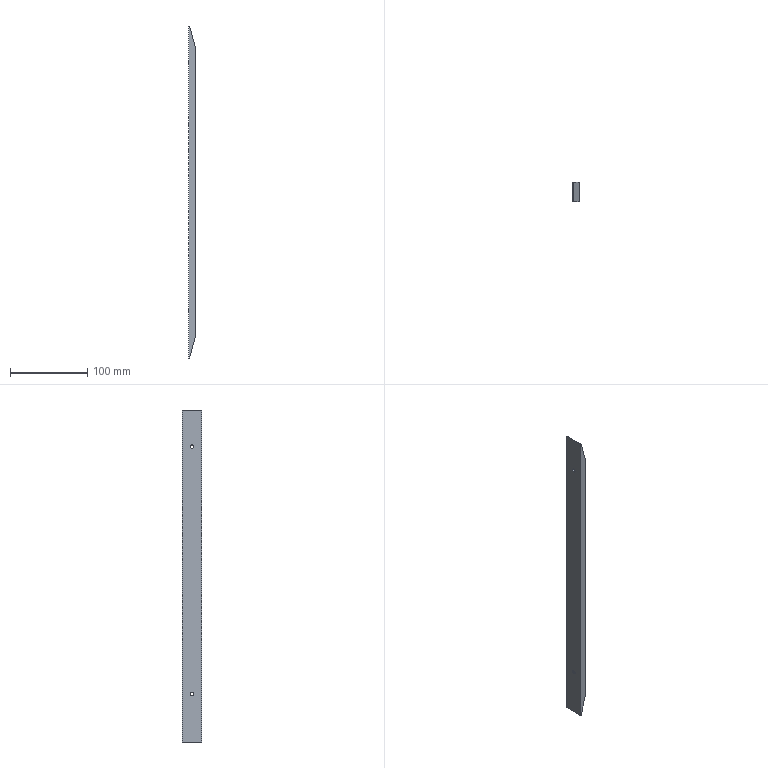Part | STEP file | 1 solid | 20 faces | box 8 x 25 x 430 mm | volume 80647 mm3 | plane 8 | cylinder 8 | cone 4 | commonest cylinder face diameters 4.5 x4 10 x4
STEP:
#1=CARTESIAN_POINT('',(0.,0.,0.));
#2=DIRECTION('',(0.,0.,1.));
#3=DIRECTION('',(1.,0.,0.));
#4=AXIS2_PLACEMENT_3D('',#1,#2,#3);
#5=CARTESIAN_POINT('',(47.75,-45.,-538.085));
#6=VERTEX_POINT('',#5);
#7=CARTESIAN_POINT('',(54.75,-45.,-511.961));
#8=VERTEX_POINT('',#7);
#9=CARTESIAN_POINT('',(47.75,-45.,-538.085));
#10=DIRECTION('',(0.2588,0.,0.9659));
#11=VECTOR('',#10,1.);
#12=LINE('',#9,#11);
#13=CARTESIAN_POINT('',(47.75,-70.,-538.085));
#14=DIRECTION('',(-0.9659,0.,0.2588));
#15=DIRECTION('',(0.,1.,0.));
#16=AXIS2_PLACEMENT_3D('',#13,#14,#15);
#17=PLANE('',#16);
#18=CARTESIAN_POINT('',(25.,0.));
#19=DIRECTION('',(0.,-1.));
#20=VECTOR('',#19,1.);
#21=LINE('',#18,#20);
#22=(GEOMETRIC_REPRESENTATION_CONTEXT(2)PARAMETRIC_REPRESENTATION_CONTEXT()REPRESENTATION_CONTEXT('',''));
#23=DEFINITIONAL_REPRESENTATION('',(#21),#22);
#24=PCURVE('',#17,#23);
#25=CARTESIAN_POINT('',(51.75,-45.,-2500.));
#26=DIRECTION('',(0.,1.,0.));
#27=DIRECTION('',(1.,0.,0.));
#28=AXIS2_PLACEMENT_3D('',#25,#26,#27);
#29=PLANE('',#28);
#30=CARTESIAN_POINT('',(-4.,-1961.915));
#31=DIRECTION('',(0.2588,-0.9659));
#32=VECTOR('',#31,1.);
#33=LINE('',#30,#32);
#34=(GEOMETRIC_REPRESENTATION_CONTEXT(2)PARAMETRIC_REPRESENTATION_CONTEXT()REPRESENTATION_CONTEXT('',''));
#35=DEFINITIONAL_REPRESENTATION('',(#33),#34);
#36=PCURVE('',#29,#35);
#37=SURFACE_CURVE('',#12,(#24,#36),.PCURVE_S1.);
#38=EDGE_CURVE('',#6,#8,#37,.T.);
#39=ORIENTED_EDGE('',*,*,#38,.T.);
#40=CARTESIAN_POINT('',(54.75,-70.,-511.961));
#41=VERTEX_POINT('',#40);
#42=CARTESIAN_POINT('',(54.75,-70.,-511.961));
#43=DIRECTION('',(0.,1.,0.));
#44=VECTOR('',#43,1.);
#45=LINE('',#42,#44);
#46=CARTESIAN_POINT('',(0.,-27.046));
#47=DIRECTION('',(1.,0.));
#48=VECTOR('',#47,1.);
#49=LINE('',#46,#48);
#50=(GEOMETRIC_REPRESENTATION_CONTEXT(2)PARAMETRIC_REPRESENTATION_CONTEXT()REPRESENTATION_CONTEXT('',''));
#51=DEFINITIONAL_REPRESENTATION('',(#49),#50);
#52=PCURVE('',#17,#51);
#53=CARTESIAN_POINT('',(54.75,0.,0.));
#54=DIRECTION('',(1.,0.,0.));
#55=DIRECTION('',(0.,1.,0.));
#56=AXIS2_PLACEMENT_3D('',#53,#54,#55);
#57=PLANE('',#56);
#58=CARTESIAN_POINT('',(-70.,-511.961));
#59=DIRECTION('',(1.,0.));
#60=VECTOR('',#59,1.);
#61=LINE('',#58,#60);
#62=(GEOMETRIC_REPRESENTATION_CONTEXT(2)PARAMETRIC_REPRESENTATION_CONTEXT()REPRESENTATION_CONTEXT('',''));
#63=DEFINITIONAL_REPRESENTATION('',(#61),#62);
#64=PCURVE('',#57,#63);
#65=SURFACE_CURVE('',#45,(#52,#64),.PCURVE_S1.);
#66=EDGE_CURVE('',#41,#8,#65,.T.);
#67=ORIENTED_EDGE('',*,*,#66,.F.);
#68=CARTESIAN_POINT('',(47.75,-70.,-538.085));
#69=VERTEX_POINT('',#68);
#70=CARTESIAN_POINT('',(47.75,-70.,-538.085));
#71=DIRECTION('',(0.2588,0.,0.9659));
#72=VECTOR('',#71,1.);
#73=LINE('',#70,#72);
#74=CARTESIAN_POINT('',(0.,0.));
#75=DIRECTION('',(0.,-1.));
#76=VECTOR('',#75,1.);
#77=LINE('',#74,#76);
#78=(GEOMETRIC_REPRESENTATION_CONTEXT(2)PARAMETRIC_REPRESENTATION_CONTEXT()REPRESENTATION_CONTEXT('',''));
#79=DEFINITIONAL_REPRESENTATION('',(#77),#78);
#80=PCURVE('',#17,#79);
#81=CARTESIAN_POINT('',(51.75,-70.,-2500.));
#82=DIRECTION('',(0.,-1.,0.));
#83=DIRECTION('',(0.,0.,-1.));
#84=AXIS2_PLACEMENT_3D('',#81,#82,#83);
#85=PLANE('',#84);
#86=CARTESIAN_POINT('',(-1961.915,-4.));
#87=DIRECTION('',(-0.9659,0.2588));
#88=VECTOR('',#87,1.);
#89=LINE('',#86,#88);
#90=(GEOMETRIC_REPRESENTATION_CONTEXT(2)PARAMETRIC_REPRESENTATION_CONTEXT()REPRESENTATION_CONTEXT('',''));
#91=DEFINITIONAL_REPRESENTATION('',(#89),#90);
#92=PCURVE('',#85,#91);
#93=SURFACE_CURVE('',#73,(#80,#92),.PCURVE_S1.);
#94=EDGE_CURVE('',#69,#41,#93,.T.);
#95=ORIENTED_EDGE('',*,*,#94,.F.);
#96=CARTESIAN_POINT('',(47.75,-70.,-538.085));
#97=DIRECTION('',(0.,1.,0.));
#98=VECTOR('',#97,1.);
#99=LINE('',#96,#98);
#100=CARTESIAN_POINT('',(0.,0.));
#101=DIRECTION('',(1.,0.));
#102=VECTOR('',#101,1.);
#103=LINE('',#100,#102);
#104=(GEOMETRIC_REPRESENTATION_CONTEXT(2)PARAMETRIC_REPRESENTATION_CONTEXT()REPRESENTATION_CONTEXT('',''));
#105=DEFINITIONAL_REPRESENTATION('',(#103),#104);
#106=PCURVE('',#17,#105);
#107=CARTESIAN_POINT('',(41.75,-45.,-538.085));
#108=DIRECTION('',(0.,0.,1.));
#109=DIRECTION('',(1.,0.,0.));
#110=AXIS2_PLACEMENT_3D('',#107,#108,#109);
#111=PLANE('',#110);
#112=CARTESIAN_POINT('',(6.,-25.));
#113=DIRECTION('',(0.,1.));
#114=VECTOR('',#113,1.);
#115=LINE('',#112,#114);
#116=(GEOMETRIC_REPRESENTATION_CONTEXT(2)PARAMETRIC_REPRESENTATION_CONTEXT()REPRESENTATION_CONTEXT('',''));
#117=DEFINITIONAL_REPRESENTATION('',(#115),#116);
#118=PCURVE('',#111,#117);
#119=SURFACE_CURVE('',#99,(#106,#118),.PCURVE_S1.);
#120=EDGE_CURVE('',#69,#6,#119,.T.);
#121=ORIENTED_EDGE('',*,*,#120,.T.);
#122=EDGE_LOOP('',(#39,#67,#95,#121));
#123=FACE_BOUND('',#122,.T.);
#124=ADVANCED_FACE('',(#123),#17,.F.);
#125=CARTESIAN_POINT('',(54.75,-45.,-134.21));
#126=VERTEX_POINT('',#125);
#127=CARTESIAN_POINT('',(47.75,-45.,-108.085));
#128=VERTEX_POINT('',#127);
#129=CARTESIAN_POINT('',(47.75,-45.,-108.085));
#130=DIRECTION('',(-0.2588,0.,0.9659));
#131=VECTOR('',#130,1.);
#132=LINE('',#129,#131);
#133=CARTESIAN_POINT('',(47.75,-70.,-108.085));
#134=DIRECTION('',(-0.9659,0.,-0.2588));
#135=DIRECTION('',(-0.2588,0.,0.9659));
#136=AXIS2_PLACEMENT_3D('',#133,#134,#135);
#137=PLANE('',#136);
#138=CARTESIAN_POINT('',(0.,25.));
#139=DIRECTION('',(1.,0.));
#140=VECTOR('',#139,1.);
#141=LINE('',#138,#140);
#142=(GEOMETRIC_REPRESENTATION_CONTEXT(2)PARAMETRIC_REPRESENTATION_CONTEXT()REPRESENTATION_CONTEXT('',''));
#143=DEFINITIONAL_REPRESENTATION('',(#141),#142);
#144=PCURVE('',#137,#143);
#145=CARTESIAN_POINT('',(-4.,-2391.915));
#146=DIRECTION('',(-0.2588,-0.9659));
#147=VECTOR('',#146,1.);
#148=LINE('',#145,#147);
#149=(GEOMETRIC_REPRESENTATION_CONTEXT(2)PARAMETRIC_REPRESENTATION_CONTEXT()REPRESENTATION_CONTEXT('',''));
#150=DEFINITIONAL_REPRESENTATION('',(#148),#149);
#151=PCURVE('',#29,#150);
#152=SURFACE_CURVE('',#132,(#144,#151),.PCURVE_S1.);
#153=EDGE_CURVE('',#126,#128,#152,.T.);
#154=ORIENTED_EDGE('',*,*,#153,.T.);
#155=CARTESIAN_POINT('',(47.75,-70.,-108.085));
#156=VERTEX_POINT('',#155);
#157=CARTESIAN_POINT('',(47.75,-70.,-108.085));
#158=DIRECTION('',(0.,1.,0.));
#159=VECTOR('',#158,1.);
#160=LINE('',#157,#159);
#161=CARTESIAN_POINT('',(0.,0.));
#162=DIRECTION('',(0.,1.));
#163=VECTOR('',#162,1.);
#164=LINE('',#161,#163);
#165=(GEOMETRIC_REPRESENTATION_CONTEXT(2)PARAMETRIC_REPRESENTATION_CONTEXT()REPRESENTATION_CONTEXT('',''));
#166=DEFINITIONAL_REPRESENTATION('',(#164),#165);
#167=PCURVE('',#137,#166);
#168=CARTESIAN_POINT('',(41.75,-45.,-108.085));
#169=DIRECTION('',(0.,0.,-1.));
#170=DIRECTION('',(0.,-1.,0.));
#171=AXIS2_PLACEMENT_3D('',#168,#169,#170);
#172=PLANE('',#171);
#173=CARTESIAN_POINT('',(25.,-6.));
#174=DIRECTION('',(-1.,0.));
#175=VECTOR('',#174,1.);
#176=LINE('',#173,#175);
#177=(GEOMETRIC_REPRESENTATION_CONTEXT(2)PARAMETRIC_REPRESENTATION_CONTEXT()REPRESENTATION_CONTEXT('',''));
#178=DEFINITIONAL_REPRESENTATION('',(#176),#177);
#179=PCURVE('',#172,#178);
#180=SURFACE_CURVE('',#160,(#167,#179),.PCURVE_S1.);
#181=EDGE_CURVE('',#156,#128,#180,.T.);
#182=ORIENTED_EDGE('',*,*,#181,.F.);
#183=CARTESIAN_POINT('',(54.75,-70.,-134.21));
#184=VERTEX_POINT('',#183);
#185=CARTESIAN_POINT('',(47.75,-70.,-108.085));
#186=DIRECTION('',(-0.2588,0.,0.9659));
#187=VECTOR('',#186,1.);
#188=LINE('',#185,#187);
#189=CARTESIAN_POINT('',(0.,0.));
#190=DIRECTION('',(1.,0.));
#191=VECTOR('',#190,1.);
#192=LINE('',#189,#191);
#193=(GEOMETRIC_REPRESENTATION_CONTEXT(2)PARAMETRIC_REPRESENTATION_CONTEXT()REPRESENTATION_CONTEXT('',''));
#194=DEFINITIONAL_REPRESENTATION('',(#192),#193);
#195=PCURVE('',#137,#194);
#196=CARTESIAN_POINT('',(-2391.915,-4.));
#197=DIRECTION('',(-0.9659,-0.2588));
#198=VECTOR('',#197,1.);
#199=LINE('',#196,#198);
#200=(GEOMETRIC_REPRESENTATION_CONTEXT(2)PARAMETRIC_REPRESENTATION_CONTEXT()REPRESENTATION_CONTEXT('',''));
#201=DEFINITIONAL_REPRESENTATION('',(#199),#200);
#202=PCURVE('',#85,#201);
#203=SURFACE_CURVE('',#188,(#195,#202),.PCURVE_S1.);
#204=EDGE_CURVE('',#184,#156,#203,.T.);
#205=ORIENTED_EDGE('',*,*,#204,.F.);
#206=CARTESIAN_POINT('',(54.75,-70.,-134.21));
#207=DIRECTION('',(0.,1.,0.));
#208=VECTOR('',#207,1.);
#209=LINE('',#206,#208);
#210=CARTESIAN_POINT('',(-27.046,0.));
#211=DIRECTION('',(0.,1.));
#212=VECTOR('',#211,1.);
#213=LINE('',#210,#212);
#214=(GEOMETRIC_REPRESENTATION_CONTEXT(2)PARAMETRIC_REPRESENTATION_CONTEXT()REPRESENTATION_CONTEXT('',''));
#215=DEFINITIONAL_REPRESENTATION('',(#213),#214);
#216=PCURVE('',#137,#215);
#217=CARTESIAN_POINT('',(-70.,-134.21));
#218=DIRECTION('',(1.,0.));
#219=VECTOR('',#218,1.);
#220=LINE('',#217,#219);
#221=(GEOMETRIC_REPRESENTATION_CONTEXT(2)PARAMETRIC_REPRESENTATION_CONTEXT()REPRESENTATION_CONTEXT('',''));
#222=DEFINITIONAL_REPRESENTATION('',(#220),#221);
#223=PCURVE('',#57,#222);
#224=SURFACE_CURVE('',#209,(#216,#223),.PCURVE_S1.);
#225=EDGE_CURVE('',#184,#126,#224,.T.);
#226=ORIENTED_EDGE('',*,*,#225,.T.);
#227=EDGE_LOOP('',(#154,#182,#205,#226));
#228=FACE_BOUND('',#227,.T.);
#229=ADVANCED_FACE('',(#228),#137,.F.);
#230=CARTESIAN_POINT('',(51.75,-57.5,-480.585));
#231=VERTEX_POINT('',#230);
#232=CARTESIAN_POINT('',(51.75,-57.5,-470.585));
#233=VERTEX_POINT('',#232);
#234=CARTESIAN_POINT('',(51.75,-57.5,-475.585));
#235=DIRECTION('',(1.,0.,0.));
#236=DIRECTION('',(0.,0.,-1.));
#237=AXIS2_PLACEMENT_3D('',#234,#235,#236);
#238=CIRCLE('',#237,5.);
#239=CARTESIAN_POINT('',(54.75,-57.5,-475.585));
#240=DIRECTION('',(-1.,0.,0.));
#241=DIRECTION('',(0.,0.,1.));
#242=AXIS2_PLACEMENT_3D('',#239,#240,#241);
#243=CYLINDRICAL_SURFACE('',#242,5.);
#244=CARTESIAN_POINT('',(3.142,3.));
#245=DIRECTION('',(-1.,0.));
#246=VECTOR('',#245,1.);
#247=LINE('',#244,#246);
#248=(GEOMETRIC_REPRESENTATION_CONTEXT(2)PARAMETRIC_REPRESENTATION_CONTEXT()REPRESENTATION_CONTEXT('',''));
#249=DEFINITIONAL_REPRESENTATION('',(#247),#248);
#250=PCURVE('',#243,#249);
#251=CARTESIAN_POINT('',(51.75,-57.5,-475.585));
#252=DIRECTION('',(1.,0.,0.));
#253=DIRECTION('',(0.,0.,-1.));
#254=AXIS2_PLACEMENT_3D('',#251,#252,#253);
#255=CONICAL_SURFACE('',#254,5.,0.7854);
#256=CARTESIAN_POINT('',(0.,0.));
#257=DIRECTION('',(1.,0.));
#258=VECTOR('',#257,1.);
#259=LINE('',#256,#258);
#260=(GEOMETRIC_REPRESENTATION_CONTEXT(2)PARAMETRIC_REPRESENTATION_CONTEXT()REPRESENTATION_CONTEXT('',''));
#261=DEFINITIONAL_REPRESENTATION('',(#259),#260);
#262=PCURVE('',#255,#261);
#263=SURFACE_CURVE('',#238,(#250,#262),.PCURVE_S1.);
#264=EDGE_CURVE('',#231,#233,#263,.T.);
#265=ORIENTED_EDGE('',*,*,#264,.T.);
#266=CARTESIAN_POINT('',(54.75,-57.5,-470.585));
#267=VERTEX_POINT('',#266);
#268=CARTESIAN_POINT('',(54.75,-57.5,-470.585));
#269=DIRECTION('',(-1.,0.,0.));
#270=VECTOR('',#269,1.);
#271=LINE('',#268,#270);
#272=CARTESIAN_POINT('',(0.,0.));
#273=DIRECTION('',(0.,1.));
#274=VECTOR('',#273,1.);
#275=LINE('',#272,#274);
#276=(GEOMETRIC_REPRESENTATION_CONTEXT(2)PARAMETRIC_REPRESENTATION_CONTEXT()REPRESENTATION_CONTEXT('',''));
#277=DEFINITIONAL_REPRESENTATION('',(#275),#276);
#278=PCURVE('',#243,#277);
#279=CARTESIAN_POINT('',(54.75,-57.5,-475.585));
#280=DIRECTION('',(-1.,0.,0.));
#281=DIRECTION('',(0.,0.,1.));
#282=AXIS2_PLACEMENT_3D('',#279,#280,#281);
#283=CYLINDRICAL_SURFACE('',#282,5.);
#284=CARTESIAN_POINT('',(6.283,0.));
#285=DIRECTION('',(0.,1.));
#286=VECTOR('',#285,1.);
#287=LINE('',#284,#286);
#288=(GEOMETRIC_REPRESENTATION_CONTEXT(2)PARAMETRIC_REPRESENTATION_CONTEXT()REPRESENTATION_CONTEXT('',''));
#289=DEFINITIONAL_REPRESENTATION('',(#287),#288);
#290=PCURVE('',#283,#289);
#291=SURFACE_CURVE('',#271,(#278,#290),.PCURVE_S1.);
#292=EDGE_CURVE('',#267,#233,#291,.T.);
#293=ORIENTED_EDGE('',*,*,#292,.F.);
#294=CARTESIAN_POINT('',(54.75,-57.5,-480.585));
#295=VERTEX_POINT('',#294);
#296=CARTESIAN_POINT('',(54.75,-57.5,-475.585));
#297=DIRECTION('',(1.,0.,0.));
#298=DIRECTION('',(0.,0.,-1.));
#299=AXIS2_PLACEMENT_3D('',#296,#297,#298);
#300=CIRCLE('',#299,5.);
#301=CARTESIAN_POINT('',(3.142,0.));
#302=DIRECTION('',(-1.,0.));
#303=VECTOR('',#302,1.);
#304=LINE('',#301,#303);
#305=(GEOMETRIC_REPRESENTATION_CONTEXT(2)PARAMETRIC_REPRESENTATION_CONTEXT()REPRESENTATION_CONTEXT('',''));
#306=DEFINITIONAL_REPRESENTATION('',(#304),#305);
#307=PCURVE('',#243,#306);
#308=CARTESIAN_POINT('',(-57.5,-475.585));
#309=DIRECTION('',(0.,-1.));
#310=AXIS2_PLACEMENT_2D('',#308,#309);
#311=CIRCLE('',#310,5.);
#312=(GEOMETRIC_REPRESENTATION_CONTEXT(2)PARAMETRIC_REPRESENTATION_CONTEXT()REPRESENTATION_CONTEXT('',''));
#313=DEFINITIONAL_REPRESENTATION('',(#311),#312);
#314=PCURVE('',#57,#313);
#315=SURFACE_CURVE('',#300,(#307,#314),.PCURVE_S1.);
#316=EDGE_CURVE('',#295,#267,#315,.T.);
#317=ORIENTED_EDGE('',*,*,#316,.F.);
#318=CARTESIAN_POINT('',(54.75,-57.5,-480.585));
#319=DIRECTION('',(-1.,0.,0.));
#320=VECTOR('',#319,1.);
#321=LINE('',#318,#320);
#322=CARTESIAN_POINT('',(3.142,0.));
#323=DIRECTION('',(0.,1.));
#324=VECTOR('',#323,1.);
#325=LINE('',#322,#324);
#326=(GEOMETRIC_REPRESENTATION_CONTEXT(2)PARAMETRIC_REPRESENTATION_CONTEXT()REPRESENTATION_CONTEXT('',''));
#327=DEFINITIONAL_REPRESENTATION('',(#325),#326);
#328=PCURVE('',#243,#327);
#329=CARTESIAN_POINT('',(3.142,0.));
#330=DIRECTION('',(0.,1.));
#331=VECTOR('',#330,1.);
#332=LINE('',#329,#331);
#333=(GEOMETRIC_REPRESENTATION_CONTEXT(2)PARAMETRIC_REPRESENTATION_CONTEXT()REPRESENTATION_CONTEXT('',''));
#334=DEFINITIONAL_REPRESENTATION('',(#332),#333);
#335=PCURVE('',#283,#334);
#336=SURFACE_CURVE('',#321,(#328,#335),.PCURVE_S1.);
#337=EDGE_CURVE('',#295,#231,#336,.T.);
#338=ORIENTED_EDGE('',*,*,#337,.T.);
#339=EDGE_LOOP('',(#265,#293,#317,#338));
#340=FACE_BOUND('',#339,.F.);
#341=ADVANCED_FACE('',(#340),#243,.F.);
#342=CARTESIAN_POINT('',(51.75,-57.5,-160.585));
#343=VERTEX_POINT('',#342);
#344=CARTESIAN_POINT('',(51.75,-57.5,-150.585));
#345=VERTEX_POINT('',#344);
#346=CARTESIAN_POINT('',(51.75,-57.5,-155.585));
#347=DIRECTION('',(1.,0.,0.));
#348=DIRECTION('',(0.,0.,-1.));
#349=AXIS2_PLACEMENT_3D('',#346,#347,#348);
#350=CIRCLE('',#349,5.);
#351=CARTESIAN_POINT('',(54.75,-57.5,-155.585));
#352=DIRECTION('',(-1.,0.,0.));
#353=DIRECTION('',(0.,0.,1.));
#354=AXIS2_PLACEMENT_3D('',#351,#352,#353);
#355=CYLINDRICAL_SURFACE('',#354,5.);
#356=CARTESIAN_POINT('',(3.142,3.));
#357=DIRECTION('',(-1.,0.));
#358=VECTOR('',#357,1.);
#359=LINE('',#356,#358);
#360=(GEOMETRIC_REPRESENTATION_CONTEXT(2)PARAMETRIC_REPRESENTATION_CONTEXT()REPRESENTATION_CONTEXT('',''));
#361=DEFINITIONAL_REPRESENTATION('',(#359),#360);
#362=PCURVE('',#355,#361);
#363=CARTESIAN_POINT('',(51.75,-57.5,-155.585));
#364=DIRECTION('',(1.,0.,0.));
#365=DIRECTION('',(0.,0.,-1.));
#366=AXIS2_PLACEMENT_3D('',#363,#364,#365);
#367=CONICAL_SURFACE('',#366,5.,0.7854);
#368=CARTESIAN_POINT('',(0.,0.));
#369=DIRECTION('',(1.,0.));
#370=VECTOR('',#369,1.);
#371=LINE('',#368,#370);
#372=(GEOMETRIC_REPRESENTATION_CONTEXT(2)PARAMETRIC_REPRESENTATION_CONTEXT()REPRESENTATION_CONTEXT('',''));
#373=DEFINITIONAL_REPRESENTATION('',(#371),#372);
#374=PCURVE('',#367,#373);
#375=SURFACE_CURVE('',#350,(#362,#374),.PCURVE_S1.);
#376=EDGE_CURVE('',#343,#345,#375,.T.);
#377=ORIENTED_EDGE('',*,*,#376,.T.);
#378=CARTESIAN_POINT('',(54.75,-57.5,-150.585));
#379=VERTEX_POINT('',#378);
#380=CARTESIAN_POINT('',(54.75,-57.5,-150.585));
#381=DIRECTION('',(-1.,0.,0.));
#382=VECTOR('',#381,1.);
#383=LINE('',#380,#382);
#384=CARTESIAN_POINT('',(0.,0.));
#385=DIRECTION('',(0.,1.));
#386=VECTOR('',#385,1.);
#387=LINE('',#384,#386);
#388=(GEOMETRIC_REPRESENTATION_CONTEXT(2)PARAMETRIC_REPRESENTATION_CONTEXT()REPRESENTATION_CONTEXT('',''));
#389=DEFINITIONAL_REPRESENTATION('',(#387),#388);
#390=PCURVE('',#355,#389);
#391=CARTESIAN_POINT('',(54.75,-57.5,-155.585));
#392=DIRECTION('',(-1.,0.,0.));
#393=DIRECTION('',(0.,0.,1.));
#394=AXIS2_PLACEMENT_3D('',#391,#392,#393);
#395=CYLINDRICAL_SURFACE('',#394,5.);
#396=CARTESIAN_POINT('',(6.283,0.));
#397=DIRECTION('',(0.,1.));
#398=VECTOR('',#397,1.);
#399=LINE('',#396,#398);
#400=(GEOMETRIC_REPRESENTATION_CONTEXT(2)PARAMETRIC_REPRESENTATION_CONTEXT()REPRESENTATION_CONTEXT('',''));
#401=DEFINITIONAL_REPRESENTATION('',(#399),#400);
#402=PCURVE('',#395,#401);
#403=SURFACE_CURVE('',#383,(#390,#402),.PCURVE_S1.);
#404=EDGE_CURVE('',#379,#345,#403,.T.);
#405=ORIENTED_EDGE('',*,*,#404,.F.);
#406=CARTESIAN_POINT('',(54.75,-57.5,-160.585));
#407=VERTEX_POINT('',#406);
#408=CARTESIAN_POINT('',(54.75,-57.5,-155.585));
#409=DIRECTION('',(1.,0.,0.));
#410=DIRECTION('',(0.,0.,-1.));
#411=AXIS2_PLACEMENT_3D('',#408,#409,#410);
#412=CIRCLE('',#411,5.);
#413=CARTESIAN_POINT('',(3.142,0.));
#414=DIRECTION('',(-1.,0.));
#415=VECTOR('',#414,1.);
#416=LINE('',#413,#415);
#417=(GEOMETRIC_REPRESENTATION_CONTEXT(2)PARAMETRIC_REPRESENTATION_CONTEXT()REPRESENTATION_CONTEXT('',''));
#418=DEFINITIONAL_REPRESENTATION('',(#416),#417);
#419=PCURVE('',#355,#418);
#420=CARTESIAN_POINT('',(-57.5,-155.585));
#421=DIRECTION('',(0.,-1.));
#422=AXIS2_PLACEMENT_2D('',#420,#421);
#423=CIRCLE('',#422,5.);
#424=(GEOMETRIC_REPRESENTATION_CONTEXT(2)PARAMETRIC_REPRESENTATION_CONTEXT()REPRESENTATION_CONTEXT('',''));
#425=DEFINITIONAL_REPRESENTATION('',(#423),#424);
#426=PCURVE('',#57,#425);
#427=SURFACE_CURVE('',#412,(#419,#426),.PCURVE_S1.);
#428=EDGE_CURVE('',#407,#379,#427,.T.);
#429=ORIENTED_EDGE('',*,*,#428,.F.);
#430=CARTESIAN_POINT('',(54.75,-57.5,-160.585));
#431=DIRECTION('',(-1.,0.,0.));
#432=VECTOR('',#431,1.);
#433=LINE('',#430,#432);
#434=CARTESIAN_POINT('',(3.142,0.));
#435=DIRECTION('',(0.,1.));
#436=VECTOR('',#435,1.);
#437=LINE('',#434,#436);
#438=(GEOMETRIC_REPRESENTATION_CONTEXT(2)PARAMETRIC_REPRESENTATION_CONTEXT()REPRESENTATION_CONTEXT('',''));
#439=DEFINITIONAL_REPRESENTATION('',(#437),#438);
#440=PCURVE('',#355,#439);
#441=CARTESIAN_POINT('',(3.142,0.));
#442=DIRECTION('',(0.,1.));
#443=VECTOR('',#442,1.);
#444=LINE('',#441,#443);
#445=(GEOMETRIC_REPRESENTATION_CONTEXT(2)PARAMETRIC_REPRESENTATION_CONTEXT()REPRESENTATION_CONTEXT('',''));
#446=DEFINITIONAL_REPRESENTATION('',(#444),#445);
#447=PCURVE('',#395,#446);
#448=SURFACE_CURVE('',#433,(#440,#447),.PCURVE_S1.);
#449=EDGE_CURVE('',#407,#343,#448,.T.);
#450=ORIENTED_EDGE('',*,*,#449,.T.);
#451=EDGE_LOOP('',(#377,#405,#429,#450));
#452=FACE_BOUND('',#451,.F.);
#453=ADVANCED_FACE('',(#452),#355,.F.);
#454=CARTESIAN_POINT('',(54.75,-57.5,-475.585));
#455=DIRECTION('',(1.,0.,0.));
#456=DIRECTION('',(0.,0.,-1.));
#457=AXIS2_PLACEMENT_3D('',#454,#455,#456);
#458=CIRCLE('',#457,5.);
#459=CARTESIAN_POINT('',(-57.5,-475.585));
#460=DIRECTION('',(0.,-1.));
#461=AXIS2_PLACEMENT_2D('',#459,#460);
#462=CIRCLE('',#461,5.);
#463=(GEOMETRIC_REPRESENTATION_CONTEXT(2)PARAMETRIC_REPRESENTATION_CONTEXT()REPRESENTATION_CONTEXT('',''));
#464=DEFINITIONAL_REPRESENTATION('',(#462),#463);
#465=PCURVE('',#57,#464);
#466=CARTESIAN_POINT('',(9.425,0.));
#467=DIRECTION('',(-1.,0.));
#468=VECTOR('',#467,1.);
#469=LINE('',#466,#468);
#470=(GEOMETRIC_REPRESENTATION_CONTEXT(2)PARAMETRIC_REPRESENTATION_CONTEXT()REPRESENTATION_CONTEXT('',''));
#471=DEFINITIONAL_REPRESENTATION('',(#469),#470);
#472=PCURVE('',#283,#471);
#473=SURFACE_CURVE('',#458,(#465,#472),.PCURVE_S1.);
#474=EDGE_CURVE('',#267,#295,#473,.T.);
#475=ORIENTED_EDGE('',*,*,#474,.F.);
#476=ORIENTED_EDGE('',*,*,#316,.F.);
#477=EDGE_LOOP('',(#475,#476));
#478=FACE_BOUND('',#477,.T.);
#479=CARTESIAN_POINT('',(54.75,-57.5,-155.585));
#480=DIRECTION('',(1.,0.,0.));
#481=DIRECTION('',(0.,0.,-1.));
#482=AXIS2_PLACEMENT_3D('',#479,#480,#481);
#483=CIRCLE('',#482,5.);
#484=CARTESIAN_POINT('',(-57.5,-155.585));
#485=DIRECTION('',(0.,-1.));
#486=AXIS2_PLACEMENT_2D('',#484,#485);
#487=CIRCLE('',#486,5.);
#488=(GEOMETRIC_REPRESENTATION_CONTEXT(2)PARAMETRIC_REPRESENTATION_CONTEXT()REPRESENTATION_CONTEXT('',''));
#489=DEFINITIONAL_REPRESENTATION('',(#487),#488);
#490=PCURVE('',#57,#489);
#491=CARTESIAN_POINT('',(9.425,0.));
#492=DIRECTION('',(-1.,0.));
#493=VECTOR('',#492,1.);
#494=LINE('',#491,#493);
#495=(GEOMETRIC_REPRESENTATION_CONTEXT(2)PARAMETRIC_REPRESENTATION_CONTEXT()REPRESENTATION_CONTEXT('',''));
#496=DEFINITIONAL_REPRESENTATION('',(#494),#495);
#497=PCURVE('',#395,#496);
#498=SURFACE_CURVE('',#483,(#490,#497),.PCURVE_S1.);
#499=EDGE_CURVE('',#379,#407,#498,.T.);
#500=ORIENTED_EDGE('',*,*,#499,.F.);
#501=ORIENTED_EDGE('',*,*,#428,.F.);
#502=EDGE_LOOP('',(#500,#501));
#503=FACE_BOUND('',#502,.T.);
#504=ORIENTED_EDGE('',*,*,#66,.T.);
#505=CARTESIAN_POINT('',(54.75,-45.,-558.085));
#506=DIRECTION('',(0.,0.,1.));
#507=VECTOR('',#506,1.);
#508=LINE('',#505,#507);
#509=CARTESIAN_POINT('',(-45.,-558.085));
#510=DIRECTION('',(0.,1.));
#511=VECTOR('',#510,1.);
#512=LINE('',#509,#511);
#513=(GEOMETRIC_REPRESENTATION_CONTEXT(2)PARAMETRIC_REPRESENTATION_CONTEXT()REPRESENTATION_CONTEXT('',''));
#514=DEFINITIONAL_REPRESENTATION('',(#512),#513);
#515=PCURVE('',#57,#514);
#516=CARTESIAN_POINT('',(3.,-1941.915));
#517=DIRECTION('',(0.,-1.));
#518=VECTOR('',#517,1.);
#519=LINE('',#516,#518);
#520=(GEOMETRIC_REPRESENTATION_CONTEXT(2)PARAMETRIC_REPRESENTATION_CONTEXT()REPRESENTATION_CONTEXT('',''));
#521=DEFINITIONAL_REPRESENTATION('',(#519),#520);
#522=PCURVE('',#29,#521);
#523=SURFACE_CURVE('',#508,(#515,#522),.PCURVE_S1.);
#524=EDGE_CURVE('',#8,#126,#523,.T.);
#525=ORIENTED_EDGE('',*,*,#524,.T.);
#526=ORIENTED_EDGE('',*,*,#225,.F.);
#527=CARTESIAN_POINT('',(54.75,-70.,-108.085));
#528=DIRECTION('',(0.,0.,-1.));
#529=VECTOR('',#528,1.);
#530=LINE('',#527,#529);
#531=CARTESIAN_POINT('',(-70.,-108.085));
#532=DIRECTION('',(0.,-1.));
#533=VECTOR('',#532,1.);
#534=LINE('',#531,#533);
#535=(GEOMETRIC_REPRESENTATION_CONTEXT(2)PARAMETRIC_REPRESENTATION_CONTEXT()REPRESENTATION_CONTEXT('',''));
#536=DEFINITIONAL_REPRESENTATION('',(#534),#535);
#537=PCURVE('',#57,#536);
#538=CARTESIAN_POINT('',(-2391.915,3.));
#539=DIRECTION('',(1.,0.));
#540=VECTOR('',#539,1.);
#541=LINE('',#538,#540);
#542=(GEOMETRIC_REPRESENTATION_CONTEXT(2)PARAMETRIC_REPRESENTATION_CONTEXT()REPRESENTATION_CONTEXT('',''));
#543=DEFINITIONAL_REPRESENTATION('',(#541),#542);
#544=PCURVE('',#85,#543);
#545=SURFACE_CURVE('',#530,(#537,#544),.PCURVE_S1.);
#546=EDGE_CURVE('',#184,#41,#545,.T.);
#547=ORIENTED_EDGE('',*,*,#546,.T.);
#548=EDGE_LOOP('',(#504,#525,#526,#547));
#549=FACE_BOUND('',#548,.T.);
#550=ADVANCED_FACE('',(#478,#503,#549),#57,.T.);
#551=ORIENTED_EDGE('',*,*,#264,.F.);
#552=CARTESIAN_POINT('',(49.,-57.5,-477.835));
#553=VERTEX_POINT('',#552);
#554=CARTESIAN_POINT('',(51.75,-57.5,-480.585));
#555=DIRECTION('',(0.7071,0.,-0.7071));
#556=VECTOR('',#555,1.);
#557=LINE('',#554,#556);
#558=CARTESIAN_POINT('',(0.,0.));
#559=DIRECTION('',(0.,1.));
#560=VECTOR('',#559,1.);
#561=LINE('',#558,#560);
#562=(GEOMETRIC_REPRESENTATION_CONTEXT(2)PARAMETRIC_REPRESENTATION_CONTEXT()REPRESENTATION_CONTEXT('',''));
#563=DEFINITIONAL_REPRESENTATION('',(#561),#562);
#564=PCURVE('',#255,#563);
#565=CARTESIAN_POINT('',(51.75,-57.5,-475.585));
#566=DIRECTION('',(1.,0.,0.));
#567=DIRECTION('',(0.,0.,-1.));
#568=AXIS2_PLACEMENT_3D('',#565,#566,#567);
#569=CONICAL_SURFACE('',#568,5.,0.7854);
#570=CARTESIAN_POINT('',(6.283,0.));
#571=DIRECTION('',(0.,1.));
#572=VECTOR('',#571,1.);
#573=LINE('',#570,#572);
#574=(GEOMETRIC_REPRESENTATION_CONTEXT(2)PARAMETRIC_REPRESENTATION_CONTEXT()REPRESENTATION_CONTEXT('',''));
#575=DEFINITIONAL_REPRESENTATION('',(#573),#574);
#576=PCURVE('',#569,#575);
#577=SURFACE_CURVE('',#557,(#564,#576),.PCURVE_S1.);
#578=EDGE_CURVE('',#553,#231,#577,.T.);
#579=ORIENTED_EDGE('',*,*,#578,.F.);
#580=CARTESIAN_POINT('',(49.,-57.5,-473.335));
#581=VERTEX_POINT('',#580);
#582=CARTESIAN_POINT('',(49.,-57.5,-475.585));
#583=DIRECTION('',(1.,0.,0.));
#584=DIRECTION('',(0.,0.,-1.));
#585=AXIS2_PLACEMENT_3D('',#582,#583,#584);
#586=CIRCLE('',#585,2.25);
#587=CARTESIAN_POINT('',(0.,-2.75));
#588=DIRECTION('',(1.,0.));
#589=VECTOR('',#588,1.);
#590=LINE('',#587,#589);
#591=(GEOMETRIC_REPRESENTATION_CONTEXT(2)PARAMETRIC_REPRESENTATION_CONTEXT()REPRESENTATION_CONTEXT('',''));
#592=DEFINITIONAL_REPRESENTATION('',(#590),#591);
#593=PCURVE('',#255,#592);
#594=CARTESIAN_POINT('',(51.75,-57.5,-475.585));
#595=DIRECTION('',(1.,0.,0.));
#596=DIRECTION('',(0.,0.,-1.));
#597=AXIS2_PLACEMENT_3D('',#594,#595,#596);
#598=CYLINDRICAL_SURFACE('',#597,2.25);
#599=CARTESIAN_POINT('',(0.,-2.75));
#600=DIRECTION('',(1.,0.));
#601=VECTOR('',#600,1.);
#602=LINE('',#599,#601);
#603=(GEOMETRIC_REPRESENTATION_CONTEXT(2)PARAMETRIC_REPRESENTATION_CONTEXT()REPRESENTATION_CONTEXT('',''));
#604=DEFINITIONAL_REPRESENTATION('',(#602),#603);
#605=PCURVE('',#598,#604);
#606=SURFACE_CURVE('',#586,(#593,#605),.PCURVE_S1.);
#607=EDGE_CURVE('',#553,#581,#606,.T.);
#608=ORIENTED_EDGE('',*,*,#607,.T.);
#609=CARTESIAN_POINT('',(51.75,-57.5,-470.585));
#610=DIRECTION('',(0.7071,0.,0.7071));
#611=VECTOR('',#610,1.);
#612=LINE('',#609,#611);
#613=CARTESIAN_POINT('',(3.142,0.));
#614=DIRECTION('',(0.,1.));
#615=VECTOR('',#614,1.);
#616=LINE('',#613,#615);
#617=(GEOMETRIC_REPRESENTATION_CONTEXT(2)PARAMETRIC_REPRESENTATION_CONTEXT()REPRESENTATION_CONTEXT('',''));
#618=DEFINITIONAL_REPRESENTATION('',(#616),#617);
#619=PCURVE('',#255,#618);
#620=CARTESIAN_POINT('',(3.142,0.));
#621=DIRECTION('',(0.,1.));
#622=VECTOR('',#621,1.);
#623=LINE('',#620,#622);
#624=(GEOMETRIC_REPRESENTATION_CONTEXT(2)PARAMETRIC_REPRESENTATION_CONTEXT()REPRESENTATION_CONTEXT('',''));
#625=DEFINITIONAL_REPRESENTATION('',(#623),#624);
#626=PCURVE('',#569,#625);
#627=SURFACE_CURVE('',#612,(#619,#626),.PCURVE_S1.);
#628=EDGE_CURVE('',#581,#233,#627,.T.);
#629=ORIENTED_EDGE('',*,*,#628,.T.);
#630=EDGE_LOOP('',(#551,#579,#608,#629));
#631=FACE_BOUND('',#630,.F.);
#632=ADVANCED_FACE('',(#631),#255,.F.);
#633=ORIENTED_EDGE('',*,*,#607,.F.);
#634=CARTESIAN_POINT('',(46.75,-57.5,-477.835));
#635=VERTEX_POINT('',#634);
#636=CARTESIAN_POINT('',(51.75,-57.5,-477.835));
#637=DIRECTION('',(1.,0.,0.));
#638=VECTOR('',#637,1.);
#639=LINE('',#636,#638);
#640=CARTESIAN_POINT('',(0.,0.));
#641=DIRECTION('',(0.,1.));
#642=VECTOR('',#641,1.);
#643=LINE('',#640,#642);
#644=(GEOMETRIC_REPRESENTATION_CONTEXT(2)PARAMETRIC_REPRESENTATION_CONTEXT()REPRESENTATION_CONTEXT('',''));
#645=DEFINITIONAL_REPRESENTATION('',(#643),#644);
#646=PCURVE('',#598,#645);
#647=CARTESIAN_POINT('',(51.75,-57.5,-475.585));
#648=DIRECTION('',(1.,0.,0.));
#649=DIRECTION('',(0.,0.,-1.));
#650=AXIS2_PLACEMENT_3D('',#647,#648,#649);
#651=CYLINDRICAL_SURFACE('',#650,2.25);
#652=CARTESIAN_POINT('',(6.283,0.));
#653=DIRECTION('',(0.,1.));
#654=VECTOR('',#653,1.);
#655=LINE('',#652,#654);
#656=(GEOMETRIC_REPRESENTATION_CONTEXT(2)PARAMETRIC_REPRESENTATION_CONTEXT()REPRESENTATION_CONTEXT('',''));
#657=DEFINITIONAL_REPRESENTATION('',(#655),#656);
#658=PCURVE('',#651,#657);
#659=SURFACE_CURVE('',#639,(#646,#658),.PCURVE_S1.);
#660=EDGE_CURVE('',#635,#553,#659,.T.);
#661=ORIENTED_EDGE('',*,*,#660,.F.);
#662=CARTESIAN_POINT('',(46.75,-57.5,-473.335));
#663=VERTEX_POINT('',#662);
#664=CARTESIAN_POINT('',(46.75,-57.5,-475.585));
#665=DIRECTION('',(1.,0.,0.));
#666=DIRECTION('',(0.,-1.,0.));
#667=AXIS2_PLACEMENT_3D('',#664,#665,#666);
#668=CIRCLE('',#667,2.25);
#669=CARTESIAN_POINT('',(-1.571,-5.));
#670=DIRECTION('',(1.,0.));
#671=VECTOR('',#670,1.);
#672=LINE('',#669,#671);
#673=(GEOMETRIC_REPRESENTATION_CONTEXT(2)PARAMETRIC_REPRESENTATION_CONTEXT()REPRESENTATION_CONTEXT('',''));
#674=DEFINITIONAL_REPRESENTATION('',(#672),#673);
#675=PCURVE('',#598,#674);
#676=CARTESIAN_POINT('',(46.75,-45.,-2500.));
#677=DIRECTION('',(-1.,0.,0.));
#678=DIRECTION('',(0.,1.,0.));
#679=AXIS2_PLACEMENT_3D('',#676,#677,#678);
#680=PLANE('',#679);
#681=CARTESIAN_POINT('',(-14.75,-2024.415));
#682=CARTESIAN_POINT('',(-14.75,-2020.518));
#683=CARTESIAN_POINT('',(-11.375,-2022.466));
#684=CARTESIAN_POINT('',(-8.,-2024.415));
#685=CARTESIAN_POINT('',(-11.375,-2026.363));
#686=CARTESIAN_POINT('',(-14.75,-2028.312));
#687=CARTESIAN_POINT('',(-14.75,-2024.415));
#688=(BOUNDED_CURVE()B_SPLINE_CURVE(2,(#681,#682,#683,#684,#685,#686,#687),.UNSPECIFIED.,.T.,.F.)B_SPLINE_CURVE_WITH_KNOTS((1,2,2,2,2,1),(-2.094,0.,2.094,4.189,6.283,8.378),.UNSPECIFIED.)CURVE()GEOMETRIC_REPRESENTATION_ITEM()RATIONAL_B_SPLINE_CURVE((1.,0.5,1.,0.5,1.,0.5,1.))REPRESENTATION_ITEM(''));
#689=(GEOMETRIC_REPRESENTATION_CONTEXT(2)PARAMETRIC_REPRESENTATION_CONTEXT()REPRESENTATION_CONTEXT('',''));
#690=DEFINITIONAL_REPRESENTATION('',(#688),#689);
#691=PCURVE('',#680,#690);
#692=SURFACE_CURVE('',#668,(#675,#691),.PCURVE_S1.);
#693=EDGE_CURVE('',#635,#663,#692,.T.);
#694=ORIENTED_EDGE('',*,*,#693,.T.);
#695=CARTESIAN_POINT('',(51.75,-57.5,-473.335));
#696=DIRECTION('',(1.,0.,0.));
#697=VECTOR('',#696,1.);
#698=LINE('',#695,#697);
#699=CARTESIAN_POINT('',(3.142,0.));
#700=DIRECTION('',(0.,1.));
#701=VECTOR('',#700,1.);
#702=LINE('',#699,#701);
#703=(GEOMETRIC_REPRESENTATION_CONTEXT(2)PARAMETRIC_REPRESENTATION_CONTEXT()REPRESENTATION_CONTEXT('',''));
#704=DEFINITIONAL_REPRESENTATION('',(#702),#703);
#705=PCURVE('',#598,#704);
#706=CARTESIAN_POINT('',(3.142,0.));
#707=DIRECTION('',(0.,1.));
#708=VECTOR('',#707,1.);
#709=LINE('',#706,#708);
#710=(GEOMETRIC_REPRESENTATION_CONTEXT(2)PARAMETRIC_REPRESENTATION_CONTEXT()REPRESENTATION_CONTEXT('',''));
#711=DEFINITIONAL_REPRESENTATION('',(#709),#710);
#712=PCURVE('',#651,#711);
#713=SURFACE_CURVE('',#698,(#705,#712),.PCURVE_S1.);
#714=EDGE_CURVE('',#663,#581,#713,.T.);
#715=ORIENTED_EDGE('',*,*,#714,.T.);
#716=EDGE_LOOP('',(#633,#661,#694,#715));
#717=FACE_BOUND('',#716,.F.);
#718=ADVANCED_FACE('',(#717),#598,.F.);
#719=ORIENTED_EDGE('',*,*,#376,.F.);
#720=CARTESIAN_POINT('',(49.,-57.5,-157.835));
#721=VERTEX_POINT('',#720);
#722=CARTESIAN_POINT('',(51.75,-57.5,-160.585));
#723=DIRECTION('',(0.7071,0.,-0.7071));
#724=VECTOR('',#723,1.);
#725=LINE('',#722,#724);
#726=CARTESIAN_POINT('',(0.,0.));
#727=DIRECTION('',(0.,1.));
#728=VECTOR('',#727,1.);
#729=LINE('',#726,#728);
#730=(GEOMETRIC_REPRESENTATION_CONTEXT(2)PARAMETRIC_REPRESENTATION_CONTEXT()REPRESENTATION_CONTEXT('',''));
#731=DEFINITIONAL_REPRESENTATION('',(#729),#730);
#732=PCURVE('',#367,#731);
#733=CARTESIAN_POINT('',(51.75,-57.5,-155.585));
#734=DIRECTION('',(1.,0.,0.));
#735=DIRECTION('',(0.,0.,-1.));
#736=AXIS2_PLACEMENT_3D('',#733,#734,#735);
#737=CONICAL_SURFACE('',#736,5.,0.7854);
#738=CARTESIAN_POINT('',(6.283,0.));
#739=DIRECTION('',(0.,1.));
#740=VECTOR('',#739,1.);
#741=LINE('',#738,#740);
#742=(GEOMETRIC_REPRESENTATION_CONTEXT(2)PARAMETRIC_REPRESENTATION_CONTEXT()REPRESENTATION_CONTEXT('',''));
#743=DEFINITIONAL_REPRESENTATION('',(#741),#742);
#744=PCURVE('',#737,#743);
#745=SURFACE_CURVE('',#725,(#732,#744),.PCURVE_S1.);
#746=EDGE_CURVE('',#721,#343,#745,.T.);
#747=ORIENTED_EDGE('',*,*,#746,.F.);
#748=CARTESIAN_POINT('',(49.,-57.5,-153.335));
#749=VERTEX_POINT('',#748);
#750=CARTESIAN_POINT('',(49.,-57.5,-155.585));
#751=DIRECTION('',(1.,0.,0.));
#752=DIRECTION('',(0.,0.,-1.));
#753=AXIS2_PLACEMENT_3D('',#750,#751,#752);
#754=CIRCLE('',#753,2.25);
#755=CARTESIAN_POINT('',(0.,-2.75));
#756=DIRECTION('',(1.,0.));
#757=VECTOR('',#756,1.);
#758=LINE('',#755,#757);
#759=(GEOMETRIC_REPRESENTATION_CONTEXT(2)PARAMETRIC_REPRESENTATION_CONTEXT()REPRESENTATION_CONTEXT('',''));
#760=DEFINITIONAL_REPRESENTATION('',(#758),#759);
#761=PCURVE('',#367,#760);
#762=CARTESIAN_POINT('',(51.75,-57.5,-155.585));
#763=DIRECTION('',(1.,0.,0.));
#764=DIRECTION('',(0.,0.,-1.));
#765=AXIS2_PLACEMENT_3D('',#762,#763,#764);
#766=CYLINDRICAL_SURFACE('',#765,2.25);
#767=CARTESIAN_POINT('',(0.,-2.75));
#768=DIRECTION('',(1.,0.));
#769=VECTOR('',#768,1.);
#770=LINE('',#767,#769);
#771=(GEOMETRIC_REPRESENTATION_CONTEXT(2)PARAMETRIC_REPRESENTATION_CONTEXT()REPRESENTATION_CONTEXT('',''));
#772=DEFINITIONAL_REPRESENTATION('',(#770),#771);
#773=PCURVE('',#766,#772);
#774=SURFACE_CURVE('',#754,(#761,#773),.PCURVE_S1.);
#775=EDGE_CURVE('',#721,#749,#774,.T.);
#776=ORIENTED_EDGE('',*,*,#775,.T.);
#777=CARTESIAN_POINT('',(51.75,-57.5,-150.585));
#778=DIRECTION('',(0.7071,0.,0.7071));
#779=VECTOR('',#778,1.);
#780=LINE('',#777,#779);
#781=CARTESIAN_POINT('',(3.142,0.));
#782=DIRECTION('',(0.,1.));
#783=VECTOR('',#782,1.);
#784=LINE('',#781,#783);
#785=(GEOMETRIC_REPRESENTATION_CONTEXT(2)PARAMETRIC_REPRESENTATION_CONTEXT()REPRESENTATION_CONTEXT('',''));
#786=DEFINITIONAL_REPRESENTATION('',(#784),#785);
#787=PCURVE('',#367,#786);
#788=CARTESIAN_POINT('',(3.142,0.));
#789=DIRECTION('',(0.,1.));
#790=VECTOR('',#789,1.);
#791=LINE('',#788,#790);
#792=(GEOMETRIC_REPRESENTATION_CONTEXT(2)PARAMETRIC_REPRESENTATION_CONTEXT()REPRESENTATION_CONTEXT('',''));
#793=DEFINITIONAL_REPRESENTATION('',(#791),#792);
#794=PCURVE('',#737,#793);
#795=SURFACE_CURVE('',#780,(#787,#794),.PCURVE_S1.);
#796=EDGE_CURVE('',#749,#345,#795,.T.);
#797=ORIENTED_EDGE('',*,*,#796,.T.);
#798=EDGE_LOOP('',(#719,#747,#776,#797));
#799=FACE_BOUND('',#798,.F.);
#800=ADVANCED_FACE('',(#799),#367,.F.);
#801=ORIENTED_EDGE('',*,*,#775,.F.);
#802=CARTESIAN_POINT('',(46.75,-57.5,-157.835));
#803=VERTEX_POINT('',#802);
#804=CARTESIAN_POINT('',(51.75,-57.5,-157.835));
#805=DIRECTION('',(1.,0.,0.));
#806=VECTOR('',#805,1.);
#807=LINE('',#804,#806);
#808=CARTESIAN_POINT('',(0.,0.));
#809=DIRECTION('',(0.,1.));
#810=VECTOR('',#809,1.);
#811=LINE('',#808,#810);
#812=(GEOMETRIC_REPRESENTATION_CONTEXT(2)PARAMETRIC_REPRESENTATION_CONTEXT()REPRESENTATION_CONTEXT('',''));
#813=DEFINITIONAL_REPRESENTATION('',(#811),#812);
#814=PCURVE('',#766,#813);
#815=CARTESIAN_POINT('',(51.75,-57.5,-155.585));
#816=DIRECTION('',(1.,0.,0.));
#817=DIRECTION('',(0.,0.,-1.));
#818=AXIS2_PLACEMENT_3D('',#815,#816,#817);
#819=CYLINDRICAL_SURFACE('',#818,2.25);
#820=CARTESIAN_POINT('',(6.283,0.));
#821=DIRECTION('',(0.,1.));
#822=VECTOR('',#821,1.);
#823=LINE('',#820,#822);
#824=(GEOMETRIC_REPRESENTATION_CONTEXT(2)PARAMETRIC_REPRESENTATION_CONTEXT()REPRESENTATION_CONTEXT('',''));
#825=DEFINITIONAL_REPRESENTATION('',(#823),#824);
#826=PCURVE('',#819,#825);
#827=SURFACE_CURVE('',#807,(#814,#826),.PCURVE_S1.);
#828=EDGE_CURVE('',#803,#721,#827,.T.);
#829=ORIENTED_EDGE('',*,*,#828,.F.);
#830=CARTESIAN_POINT('',(46.75,-57.5,-153.335));
#831=VERTEX_POINT('',#830);
#832=CARTESIAN_POINT('',(46.75,-57.5,-155.585));
#833=DIRECTION('',(1.,0.,0.));
#834=DIRECTION('',(0.,-1.,0.));
#835=AXIS2_PLACEMENT_3D('',#832,#833,#834);
#836=CIRCLE('',#835,2.25);
#837=CARTESIAN_POINT('',(-1.571,-5.));
#838=DIRECTION('',(1.,0.));
#839=VECTOR('',#838,1.);
#840=LINE('',#837,#839);
#841=(GEOMETRIC_REPRESENTATION_CONTEXT(2)PARAMETRIC_REPRESENTATION_CONTEXT()REPRESENTATION_CONTEXT('',''));
#842=DEFINITIONAL_REPRESENTATION('',(#840),#841);
#843=PCURVE('',#766,#842);
#844=CARTESIAN_POINT('',(-14.75,-2344.415));
#845=CARTESIAN_POINT('',(-14.75,-2340.518));
#846=CARTESIAN_POINT('',(-11.375,-2342.466));
#847=CARTESIAN_POINT('',(-8.,-2344.415));
#848=CARTESIAN_POINT('',(-11.375,-2346.363));
#849=CARTESIAN_POINT('',(-14.75,-2348.312));
#850=CARTESIAN_POINT('',(-14.75,-2344.415));
#851=(BOUNDED_CURVE()B_SPLINE_CURVE(2,(#844,#845,#846,#847,#848,#849,#850),.UNSPECIFIED.,.T.,.F.)B_SPLINE_CURVE_WITH_KNOTS((1,2,2,2,2,1),(-2.094,0.,2.094,4.189,6.283,8.378),.UNSPECIFIED.)CURVE()GEOMETRIC_REPRESENTATION_ITEM()RATIONAL_B_SPLINE_CURVE((1.,0.5,1.,0.5,1.,0.5,1.))REPRESENTATION_ITEM(''));
#852=(GEOMETRIC_REPRESENTATION_CONTEXT(2)PARAMETRIC_REPRESENTATION_CONTEXT()REPRESENTATION_CONTEXT('',''));
#853=DEFINITIONAL_REPRESENTATION('',(#851),#852);
#854=PCURVE('',#680,#853);
#855=SURFACE_CURVE('',#836,(#843,#854),.PCURVE_S1.);
#856=EDGE_CURVE('',#803,#831,#855,.T.);
#857=ORIENTED_EDGE('',*,*,#856,.T.);
#858=CARTESIAN_POINT('',(51.75,-57.5,-153.335));
#859=DIRECTION('',(1.,0.,0.));
#860=VECTOR('',#859,1.);
#861=LINE('',#858,#860);
#862=CARTESIAN_POINT('',(3.142,0.));
#863=DIRECTION('',(0.,1.));
#864=VECTOR('',#863,1.);
#865=LINE('',#862,#864);
#866=(GEOMETRIC_REPRESENTATION_CONTEXT(2)PARAMETRIC_REPRESENTATION_CONTEXT()REPRESENTATION_CONTEXT('',''));
#867=DEFINITIONAL_REPRESENTATION('',(#865),#866);
#868=PCURVE('',#766,#867);
#869=CARTESIAN_POINT('',(3.142,0.));
#870=DIRECTION('',(0.,1.));
#871=VECTOR('',#870,1.);
#872=LINE('',#869,#871);
#873=(GEOMETRIC_REPRESENTATION_CONTEXT(2)PARAMETRIC_REPRESENTATION_CONTEXT()REPRESENTATION_CONTEXT('',''));
#874=DEFINITIONAL_REPRESENTATION('',(#872),#873);
#875=PCURVE('',#819,#874);
#876=SURFACE_CURVE('',#861,(#868,#875),.PCURVE_S1.);
#877=EDGE_CURVE('',#831,#749,#876,.T.);
#878=ORIENTED_EDGE('',*,*,#877,.T.);
#879=EDGE_LOOP('',(#801,#829,#857,#878));
#880=FACE_BOUND('',#879,.F.);
#881=ADVANCED_FACE('',(#880),#766,.F.);
#882=CARTESIAN_POINT('',(46.75,-45.,-538.085));
#883=VERTEX_POINT('',#882);
#884=CARTESIAN_POINT('',(41.75,-45.,-538.085));
#885=DIRECTION('',(1.,0.,0.));
#886=VECTOR('',#885,1.);
#887=LINE('',#884,#886);
#888=CARTESIAN_POINT('',(0.,0.));
#889=DIRECTION('',(1.,0.));
#890=VECTOR('',#889,1.);
#891=LINE('',#888,#890);
#892=(GEOMETRIC_REPRESENTATION_CONTEXT(2)PARAMETRIC_REPRESENTATION_CONTEXT()REPRESENTATION_CONTEXT('',''));
#893=DEFINITIONAL_REPRESENTATION('',(#891),#892);
#894=PCURVE('',#111,#893);
#895=CARTESIAN_POINT('',(-10.,-1961.915));
#896=DIRECTION('',(1.,0.));
#897=VECTOR('',#896,1.);
#898=LINE('',#895,#897);
#899=(GEOMETRIC_REPRESENTATION_CONTEXT(2)PARAMETRIC_REPRESENTATION_CONTEXT()REPRESENTATION_CONTEXT('',''));
#900=DEFINITIONAL_REPRESENTATION('',(#898),#899);
#901=PCURVE('',#29,#900);
#902=SURFACE_CURVE('',#887,(#894,#901),.PCURVE_S1.);
#903=EDGE_CURVE('',#883,#6,#902,.T.);
#904=ORIENTED_EDGE('',*,*,#903,.T.);
#905=ORIENTED_EDGE('',*,*,#120,.F.);
#906=CARTESIAN_POINT('',(46.75,-70.,-538.085));
#907=VERTEX_POINT('',#906);
#908=CARTESIAN_POINT('',(41.75,-70.,-538.085));
#909=DIRECTION('',(1.,0.,0.));
#910=VECTOR('',#909,1.);
#911=LINE('',#908,#910);
#912=CARTESIAN_POINT('',(0.,-25.));
#913=DIRECTION('',(1.,0.));
#914=VECTOR('',#913,1.);
#915=LINE('',#912,#914);
#916=(GEOMETRIC_REPRESENTATION_CONTEXT(2)PARAMETRIC_REPRESENTATION_CONTEXT()REPRESENTATION_CONTEXT('',''));
#917=DEFINITIONAL_REPRESENTATION('',(#915),#916);
#918=PCURVE('',#111,#917);
#919=CARTESIAN_POINT('',(-1961.915,-10.));
#920=DIRECTION('',(0.,1.));
#921=VECTOR('',#920,1.);
#922=LINE('',#919,#921);
#923=(GEOMETRIC_REPRESENTATION_CONTEXT(2)PARAMETRIC_REPRESENTATION_CONTEXT()REPRESENTATION_CONTEXT('',''));
#924=DEFINITIONAL_REPRESENTATION('',(#922),#923);
#925=PCURVE('',#85,#924);
#926=SURFACE_CURVE('',#911,(#918,#925),.PCURVE_S1.);
#927=EDGE_CURVE('',#907,#69,#926,.T.);
#928=ORIENTED_EDGE('',*,*,#927,.F.);
#929=CARTESIAN_POINT('',(46.75,-45.,-538.085));
#930=DIRECTION('',(0.,-1.,0.));
#931=VECTOR('',#930,1.);
#932=LINE('',#929,#931);
#933=CARTESIAN_POINT('',(5.,0.));
#934=DIRECTION('',(0.,-1.));
#935=VECTOR('',#934,1.);
#936=LINE('',#933,#935);
#937=(GEOMETRIC_REPRESENTATION_CONTEXT(2)PARAMETRIC_REPRESENTATION_CONTEXT()REPRESENTATION_CONTEXT('',''));
#938=DEFINITIONAL_REPRESENTATION('',(#936),#937);
#939=PCURVE('',#111,#938);
#940=CARTESIAN_POINT('',(0.,-1961.915));
#941=DIRECTION('',(-1.,0.));
#942=VECTOR('',#941,1.);
#943=LINE('',#940,#942);
#944=(GEOMETRIC_REPRESENTATION_CONTEXT(2)PARAMETRIC_REPRESENTATION_CONTEXT()REPRESENTATION_CONTEXT('',''));
#945=DEFINITIONAL_REPRESENTATION('',(#943),#944);
#946=PCURVE('',#680,#945);
#947=SURFACE_CURVE('',#932,(#939,#946),.PCURVE_S1.);
#948=EDGE_CURVE('',#883,#907,#947,.T.);
#949=ORIENTED_EDGE('',*,*,#948,.F.);
#950=EDGE_LOOP('',(#904,#905,#928,#949));
#951=FACE_BOUND('',#950,.T.);
#952=ADVANCED_FACE('',(#951),#111,.F.);
#953=CARTESIAN_POINT('',(46.75,-70.,-108.085));
#954=VERTEX_POINT('',#953);
#955=CARTESIAN_POINT('',(41.75,-70.,-108.085));
#956=DIRECTION('',(1.,0.,0.));
#957=VECTOR('',#956,1.);
#958=LINE('',#955,#957);
#959=CARTESIAN_POINT('',(25.,0.));
#960=DIRECTION('',(0.,-1.));
#961=VECTOR('',#960,1.);
#962=LINE('',#959,#961);
#963=(GEOMETRIC_REPRESENTATION_CONTEXT(2)PARAMETRIC_REPRESENTATION_CONTEXT()REPRESENTATION_CONTEXT('',''));
#964=DEFINITIONAL_REPRESENTATION('',(#962),#963);
#965=PCURVE('',#172,#964);
#966=CARTESIAN_POINT('',(-2391.915,-10.));
#967=DIRECTION('',(0.,1.));
#968=VECTOR('',#967,1.);
#969=LINE('',#966,#968);
#970=(GEOMETRIC_REPRESENTATION_CONTEXT(2)PARAMETRIC_REPRESENTATION_CONTEXT()REPRESENTATION_CONTEXT('',''));
#971=DEFINITIONAL_REPRESENTATION('',(#969),#970);
#972=PCURVE('',#85,#971);
#973=SURFACE_CURVE('',#958,(#965,#972),.PCURVE_S1.);
#974=EDGE_CURVE('',#954,#156,#973,.T.);
#975=ORIENTED_EDGE('',*,*,#974,.T.);
#976=ORIENTED_EDGE('',*,*,#181,.T.);
#977=CARTESIAN_POINT('',(46.75,-45.,-108.085));
#978=VERTEX_POINT('',#977);
#979=CARTESIAN_POINT('',(41.75,-45.,-108.085));
#980=DIRECTION('',(1.,0.,0.));
#981=VECTOR('',#980,1.);
#982=LINE('',#979,#981);
#983=CARTESIAN_POINT('',(0.,0.));
#984=DIRECTION('',(0.,-1.));
#985=VECTOR('',#984,1.);
#986=LINE('',#983,#985);
#987=(GEOMETRIC_REPRESENTATION_CONTEXT(2)PARAMETRIC_REPRESENTATION_CONTEXT()REPRESENTATION_CONTEXT('',''));
#988=DEFINITIONAL_REPRESENTATION('',(#986),#987);
#989=PCURVE('',#172,#988);
#990=CARTESIAN_POINT('',(-10.,-2391.915));
#991=DIRECTION('',(1.,0.));
#992=VECTOR('',#991,1.);
#993=LINE('',#990,#992);
#994=(GEOMETRIC_REPRESENTATION_CONTEXT(2)PARAMETRIC_REPRESENTATION_CONTEXT()REPRESENTATION_CONTEXT('',''));
#995=DEFINITIONAL_REPRESENTATION('',(#993),#994);
#996=PCURVE('',#29,#995);
#997=SURFACE_CURVE('',#982,(#989,#996),.PCURVE_S1.);
#998=EDGE_CURVE('',#978,#128,#997,.T.);
#999=ORIENTED_EDGE('',*,*,#998,.F.);
#1000=CARTESIAN_POINT('',(46.75,-45.,-108.085));
#1001=DIRECTION('',(0.,1.,0.));
#1002=VECTOR('',#1001,1.);
#1003=LINE('',#1000,#1002);
#1004=CARTESIAN_POINT('',(0.,-5.));
#1005=DIRECTION('',(-1.,0.));
#1006=VECTOR('',#1005,1.);
#1007=LINE('',#1004,#1006);
#1008=(GEOMETRIC_REPRESENTATION_CONTEXT(2)PARAMETRIC_REPRESENTATION_CONTEXT()REPRESENTATION_CONTEXT('',''));
#1009=DEFINITIONAL_REPRESENTATION('',(#1007),#1008);
#1010=PCURVE('',#172,#1009);
#1011=CARTESIAN_POINT('',(0.,-2391.915));
#1012=DIRECTION('',(1.,0.));
#1013=VECTOR('',#1012,1.);
#1014=LINE('',#1011,#1013);
#1015=(GEOMETRIC_REPRESENTATION_CONTEXT(2)PARAMETRIC_REPRESENTATION_CONTEXT()REPRESENTATION_CONTEXT('',''));
#1016=DEFINITIONAL_REPRESENTATION('',(#1014),#1015);
#1017=PCURVE('',#680,#1016);
#1018=SURFACE_CURVE('',#1003,(#1010,#1017),.PCURVE_S1.);
#1019=EDGE_CURVE('',#954,#978,#1018,.T.);
#1020=ORIENTED_EDGE('',*,*,#1019,.F.);
#1021=EDGE_LOOP('',(#975,#976,#999,#1020));
#1022=FACE_BOUND('',#1021,.T.);
#1023=ADVANCED_FACE('',(#1022),#172,.F.);
#1024=ORIENTED_EDGE('',*,*,#856,.T.);
#1025=CARTESIAN_POINT('',(46.75,-57.5,-155.585));
#1026=DIRECTION('',(1.,0.,0.));
#1027=DIRECTION('',(0.,-1.,0.));
#1028=AXIS2_PLACEMENT_3D('',#1025,#1026,#1027);
#1029=CIRCLE('',#1028,2.25);
#1030=CARTESIAN_POINT('',(-14.75,-2344.415));
#1031=CARTESIAN_POINT('',(-14.75,-2340.518));
#1032=CARTESIAN_POINT('',(-11.375,-2342.466));
#1033=CARTESIAN_POINT('',(-8.,-2344.415));
#1034=CARTESIAN_POINT('',(-11.375,-2346.363));
#1035=CARTESIAN_POINT('',(-14.75,-2348.312));
#1036=CARTESIAN_POINT('',(-14.75,-2344.415));
#1037=(BOUNDED_CURVE()B_SPLINE_CURVE(2,(#1030,#1031,#1032,#1033,#1034,#1035,#1036),.UNSPECIFIED.,.T.,.F.)B_SPLINE_CURVE_WITH_KNOTS((1,2,2,2,2,1),(-2.094,0.,2.094,4.189,6.283,8.378),.UNSPECIFIED.)CURVE()GEOMETRIC_REPRESENTATION_ITEM()RATIONAL_B_SPLINE_CURVE((1.,0.5,1.,0.5,1.,0.5,1.))REPRESENTATION_ITEM(''));
#1038=(GEOMETRIC_REPRESENTATION_CONTEXT(2)PARAMETRIC_REPRESENTATION_CONTEXT()REPRESENTATION_CONTEXT('',''));
#1039=DEFINITIONAL_REPRESENTATION('',(#1037),#1038);
#1040=PCURVE('',#680,#1039);
#1041=CARTESIAN_POINT('',(-1.571,-5.));
#1042=DIRECTION('',(1.,0.));
#1043=VECTOR('',#1042,1.);
#1044=LINE('',#1041,#1043);
#1045=(GEOMETRIC_REPRESENTATION_CONTEXT(2)PARAMETRIC_REPRESENTATION_CONTEXT()REPRESENTATION_CONTEXT('',''));
#1046=DEFINITIONAL_REPRESENTATION('',(#1044),#1045);
#1047=PCURVE('',#819,#1046);
#1048=SURFACE_CURVE('',#1029,(#1040,#1047),.PCURVE_S1.);
#1049=EDGE_CURVE('',#831,#803,#1048,.T.);
#1050=ORIENTED_EDGE('',*,*,#1049,.T.);
#1051=EDGE_LOOP('',(#1024,#1050));
#1052=FACE_BOUND('',#1051,.T.);
#1053=ORIENTED_EDGE('',*,*,#693,.T.);
#1054=CARTESIAN_POINT('',(46.75,-57.5,-475.585));
#1055=DIRECTION('',(1.,0.,0.));
#1056=DIRECTION('',(0.,-1.,0.));
#1057=AXIS2_PLACEMENT_3D('',#1054,#1055,#1056);
#1058=CIRCLE('',#1057,2.25);
#1059=CARTESIAN_POINT('',(-14.75,-2024.415));
#1060=CARTESIAN_POINT('',(-14.75,-2020.518));
#1061=CARTESIAN_POINT('',(-11.375,-2022.466));
#1062=CARTESIAN_POINT('',(-8.,-2024.415));
#1063=CARTESIAN_POINT('',(-11.375,-2026.363));
#1064=CARTESIAN_POINT('',(-14.75,-2028.312));
#1065=CARTESIAN_POINT('',(-14.75,-2024.415));
#1066=(BOUNDED_CURVE()B_SPLINE_CURVE(2,(#1059,#1060,#1061,#1062,#1063,#1064,#1065),.UNSPECIFIED.,.T.,.F.)B_SPLINE_CURVE_WITH_KNOTS((1,2,2,2,2,1),(-2.094,0.,2.094,4.189,6.283,8.378),.UNSPECIFIED.)CURVE()GEOMETRIC_REPRESENTATION_ITEM()RATIONAL_B_SPLINE_CURVE((1.,0.5,1.,0.5,1.,0.5,1.))REPRESENTATION_ITEM(''));
#1067=(GEOMETRIC_REPRESENTATION_CONTEXT(2)PARAMETRIC_REPRESENTATION_CONTEXT()REPRESENTATION_CONTEXT('',''));
#1068=DEFINITIONAL_REPRESENTATION('',(#1066),#1067);
#1069=PCURVE('',#680,#1068);
#1070=CARTESIAN_POINT('',(-1.571,-5.));
#1071=DIRECTION('',(1.,0.));
#1072=VECTOR('',#1071,1.);
#1073=LINE('',#1070,#1072);
#1074=(GEOMETRIC_REPRESENTATION_CONTEXT(2)PARAMETRIC_REPRESENTATION_CONTEXT()REPRESENTATION_CONTEXT('',''));
#1075=DEFINITIONAL_REPRESENTATION('',(#1073),#1074);
#1076=PCURVE('',#651,#1075);
#1077=SURFACE_CURVE('',#1058,(#1069,#1076),.PCURVE_S1.);
#1078=EDGE_CURVE('',#663,#635,#1077,.T.);
#1079=ORIENTED_EDGE('',*,*,#1078,.T.);
#1080=EDGE_LOOP('',(#1053,#1079));
#1081=FACE_BOUND('',#1080,.T.);
#1082=ORIENTED_EDGE('',*,*,#948,.T.);
#1083=CARTESIAN_POINT('',(46.75,-70.,-2500.));
#1084=DIRECTION('',(0.,0.,-1.));
#1085=VECTOR('',#1084,1.);
#1086=LINE('',#1083,#1085);
#1087=CARTESIAN_POINT('',(-25.,0.));
#1088=DIRECTION('',(0.,1.));
#1089=VECTOR('',#1088,1.);
#1090=LINE('',#1087,#1089);
#1091=(GEOMETRIC_REPRESENTATION_CONTEXT(2)PARAMETRIC_REPRESENTATION_CONTEXT()REPRESENTATION_CONTEXT('',''));
#1092=DEFINITIONAL_REPRESENTATION('',(#1090),#1091);
#1093=PCURVE('',#680,#1092);
#1094=CARTESIAN_POINT('',(0.,-5.));
#1095=DIRECTION('',(1.,0.));
#1096=VECTOR('',#1095,1.);
#1097=LINE('',#1094,#1096);
#1098=(GEOMETRIC_REPRESENTATION_CONTEXT(2)PARAMETRIC_REPRESENTATION_CONTEXT()REPRESENTATION_CONTEXT('',''));
#1099=DEFINITIONAL_REPRESENTATION('',(#1097),#1098);
#1100=PCURVE('',#85,#1099);
#1101=SURFACE_CURVE('',#1086,(#1093,#1100),.PCURVE_S1.);
#1102=EDGE_CURVE('',#954,#907,#1101,.T.);
#1103=ORIENTED_EDGE('',*,*,#1102,.F.);
#1104=ORIENTED_EDGE('',*,*,#1019,.T.);
#1105=CARTESIAN_POINT('',(46.75,-45.,-2500.));
#1106=DIRECTION('',(0.,0.,1.));
#1107=VECTOR('',#1106,1.);
#1108=LINE('',#1105,#1107);
#1109=CARTESIAN_POINT('',(0.,0.));
#1110=DIRECTION('',(0.,-1.));
#1111=VECTOR('',#1110,1.);
#1112=LINE('',#1109,#1111);
#1113=(GEOMETRIC_REPRESENTATION_CONTEXT(2)PARAMETRIC_REPRESENTATION_CONTEXT()REPRESENTATION_CONTEXT('',''));
#1114=DEFINITIONAL_REPRESENTATION('',(#1112),#1113);
#1115=PCURVE('',#680,#1114);
#1116=CARTESIAN_POINT('',(-5.,0.));
#1117=DIRECTION('',(0.,-1.));
#1118=VECTOR('',#1117,1.);
#1119=LINE('',#1116,#1118);
#1120=(GEOMETRIC_REPRESENTATION_CONTEXT(2)PARAMETRIC_REPRESENTATION_CONTEXT()REPRESENTATION_CONTEXT('',''));
#1121=DEFINITIONAL_REPRESENTATION('',(#1119),#1120);
#1122=PCURVE('',#29,#1121);
#1123=SURFACE_CURVE('',#1108,(#1115,#1122),.PCURVE_S1.);
#1124=EDGE_CURVE('',#883,#978,#1123,.T.);
#1125=ORIENTED_EDGE('',*,*,#1124,.F.);
#1126=EDGE_LOOP('',(#1082,#1103,#1104,#1125));
#1127=FACE_BOUND('',#1126,.T.);
#1128=ADVANCED_FACE('',(#1052,#1081,#1127),#680,.T.);
#1129=ORIENTED_EDGE('',*,*,#94,.T.);
#1130=ORIENTED_EDGE('',*,*,#546,.F.);
#1131=ORIENTED_EDGE('',*,*,#204,.T.);
#1132=ORIENTED_EDGE('',*,*,#974,.F.);
#1133=ORIENTED_EDGE('',*,*,#1102,.T.);
#1134=ORIENTED_EDGE('',*,*,#927,.T.);
#1135=EDGE_LOOP('',(#1129,#1130,#1131,#1132,#1133,#1134));
#1136=FACE_BOUND('',#1135,.T.);
#1137=ADVANCED_FACE('',(#1136),#85,.T.);
#1138=ORIENTED_EDGE('',*,*,#38,.F.);
#1139=ORIENTED_EDGE('',*,*,#903,.F.);
#1140=ORIENTED_EDGE('',*,*,#1124,.T.);
#1141=ORIENTED_EDGE('',*,*,#998,.T.);
#1142=ORIENTED_EDGE('',*,*,#153,.F.);
#1143=ORIENTED_EDGE('',*,*,#524,.F.);
#1144=EDGE_LOOP('',(#1138,#1139,#1140,#1141,#1142,#1143));
#1145=FACE_BOUND('',#1144,.T.);
#1146=ADVANCED_FACE('',(#1145),#29,.T.);
#1147=ORIENTED_EDGE('',*,*,#828,.T.);
#1148=CARTESIAN_POINT('',(49.,-57.5,-155.585));
#1149=DIRECTION('',(1.,0.,0.));
#1150=DIRECTION('',(0.,0.,-1.));
#1151=AXIS2_PLACEMENT_3D('',#1148,#1149,#1150);
#1152=CIRCLE('',#1151,2.25);
#1153=CARTESIAN_POINT('',(0.,-2.75));
#1154=DIRECTION('',(1.,0.));
#1155=VECTOR('',#1154,1.);
#1156=LINE('',#1153,#1155);
#1157=(GEOMETRIC_REPRESENTATION_CONTEXT(2)PARAMETRIC_REPRESENTATION_CONTEXT()REPRESENTATION_CONTEXT('',''));
#1158=DEFINITIONAL_REPRESENTATION('',(#1156),#1157);
#1159=PCURVE('',#819,#1158);
#1160=CARTESIAN_POINT('',(0.,-2.75));
#1161=DIRECTION('',(1.,0.));
#1162=VECTOR('',#1161,1.);
#1163=LINE('',#1160,#1162);
#1164=(GEOMETRIC_REPRESENTATION_CONTEXT(2)PARAMETRIC_REPRESENTATION_CONTEXT()REPRESENTATION_CONTEXT('',''));
#1165=DEFINITIONAL_REPRESENTATION('',(#1163),#1164);
#1166=PCURVE('',#737,#1165);
#1167=SURFACE_CURVE('',#1152,(#1159,#1166),.PCURVE_S1.);
#1168=EDGE_CURVE('',#749,#721,#1167,.T.);
#1169=ORIENTED_EDGE('',*,*,#1168,.F.);
#1170=ORIENTED_EDGE('',*,*,#877,.F.);
#1171=ORIENTED_EDGE('',*,*,#1049,.T.);
#1172=EDGE_LOOP('',(#1147,#1169,#1170,#1171));
#1173=FACE_BOUND('',#1172,.F.);
#1174=ADVANCED_FACE('',(#1173),#819,.F.);
#1175=ORIENTED_EDGE('',*,*,#746,.T.);
#1176=CARTESIAN_POINT('',(51.75,-57.5,-155.585));
#1177=DIRECTION('',(1.,0.,0.));
#1178=DIRECTION('',(0.,0.,-1.));
#1179=AXIS2_PLACEMENT_3D('',#1176,#1177,#1178);
#1180=CIRCLE('',#1179,5.);
#1181=CARTESIAN_POINT('',(0.,0.));
#1182=DIRECTION('',(1.,0.));
#1183=VECTOR('',#1182,1.);
#1184=LINE('',#1181,#1183);
#1185=(GEOMETRIC_REPRESENTATION_CONTEXT(2)PARAMETRIC_REPRESENTATION_CONTEXT()REPRESENTATION_CONTEXT('',''));
#1186=DEFINITIONAL_REPRESENTATION('',(#1184),#1185);
#1187=PCURVE('',#737,#1186);
#1188=CARTESIAN_POINT('',(9.425,3.));
#1189=DIRECTION('',(-1.,0.));
#1190=VECTOR('',#1189,1.);
#1191=LINE('',#1188,#1190);
#1192=(GEOMETRIC_REPRESENTATION_CONTEXT(2)PARAMETRIC_REPRESENTATION_CONTEXT()REPRESENTATION_CONTEXT('',''));
#1193=DEFINITIONAL_REPRESENTATION('',(#1191),#1192);
#1194=PCURVE('',#395,#1193);
#1195=SURFACE_CURVE('',#1180,(#1187,#1194),.PCURVE_S1.);
#1196=EDGE_CURVE('',#345,#343,#1195,.T.);
#1197=ORIENTED_EDGE('',*,*,#1196,.F.);
#1198=ORIENTED_EDGE('',*,*,#796,.F.);
#1199=ORIENTED_EDGE('',*,*,#1168,.T.);
#1200=EDGE_LOOP('',(#1175,#1197,#1198,#1199));
#1201=FACE_BOUND('',#1200,.F.);
#1202=ADVANCED_FACE('',(#1201),#737,.F.);
#1203=ORIENTED_EDGE('',*,*,#660,.T.);
#1204=CARTESIAN_POINT('',(49.,-57.5,-475.585));
#1205=DIRECTION('',(1.,0.,0.));
#1206=DIRECTION('',(0.,0.,-1.));
#1207=AXIS2_PLACEMENT_3D('',#1204,#1205,#1206);
#1208=CIRCLE('',#1207,2.25);
#1209=CARTESIAN_POINT('',(0.,-2.75));
#1210=DIRECTION('',(1.,0.));
#1211=VECTOR('',#1210,1.);
#1212=LINE('',#1209,#1211);
#1213=(GEOMETRIC_REPRESENTATION_CONTEXT(2)PARAMETRIC_REPRESENTATION_CONTEXT()REPRESENTATION_CONTEXT('',''));
#1214=DEFINITIONAL_REPRESENTATION('',(#1212),#1213);
#1215=PCURVE('',#651,#1214);
#1216=CARTESIAN_POINT('',(0.,-2.75));
#1217=DIRECTION('',(1.,0.));
#1218=VECTOR('',#1217,1.);
#1219=LINE('',#1216,#1218);
#1220=(GEOMETRIC_REPRESENTATION_CONTEXT(2)PARAMETRIC_REPRESENTATION_CONTEXT()REPRESENTATION_CONTEXT('',''));
#1221=DEFINITIONAL_REPRESENTATION('',(#1219),#1220);
#1222=PCURVE('',#569,#1221);
#1223=SURFACE_CURVE('',#1208,(#1215,#1222),.PCURVE_S1.);
#1224=EDGE_CURVE('',#581,#553,#1223,.T.);
#1225=ORIENTED_EDGE('',*,*,#1224,.F.);
#1226=ORIENTED_EDGE('',*,*,#714,.F.);
#1227=ORIENTED_EDGE('',*,*,#1078,.T.);
#1228=EDGE_LOOP('',(#1203,#1225,#1226,#1227));
#1229=FACE_BOUND('',#1228,.F.);
#1230=ADVANCED_FACE('',(#1229),#651,.F.);
#1231=ORIENTED_EDGE('',*,*,#578,.T.);
#1232=CARTESIAN_POINT('',(51.75,-57.5,-475.585));
#1233=DIRECTION('',(1.,0.,0.));
#1234=DIRECTION('',(0.,0.,-1.));
#1235=AXIS2_PLACEMENT_3D('',#1232,#1233,#1234);
#1236=CIRCLE('',#1235,5.);
#1237=CARTESIAN_POINT('',(0.,0.));
#1238=DIRECTION('',(1.,0.));
#1239=VECTOR('',#1238,1.);
#1240=LINE('',#1237,#1239);
#1241=(GEOMETRIC_REPRESENTATION_CONTEXT(2)PARAMETRIC_REPRESENTATION_CONTEXT()REPRESENTATION_CONTEXT('',''));
#1242=DEFINITIONAL_REPRESENTATION('',(#1240),#1241);
#1243=PCURVE('',#569,#1242);
#1244=CARTESIAN_POINT('',(9.425,3.));
#1245=DIRECTION('',(-1.,0.));
#1246=VECTOR('',#1245,1.);
#1247=LINE('',#1244,#1246);
#1248=(GEOMETRIC_REPRESENTATION_CONTEXT(2)PARAMETRIC_REPRESENTATION_CONTEXT()REPRESENTATION_CONTEXT('',''));
#1249=DEFINITIONAL_REPRESENTATION('',(#1247),#1248);
#1250=PCURVE('',#283,#1249);
#1251=SURFACE_CURVE('',#1236,(#1243,#1250),.PCURVE_S1.);
#1252=EDGE_CURVE('',#233,#231,#1251,.T.);
#1253=ORIENTED_EDGE('',*,*,#1252,.F.);
#1254=ORIENTED_EDGE('',*,*,#628,.F.);
#1255=ORIENTED_EDGE('',*,*,#1224,.T.);
#1256=EDGE_LOOP('',(#1231,#1253,#1254,#1255));
#1257=FACE_BOUND('',#1256,.F.);
#1258=ADVANCED_FACE('',(#1257),#569,.F.);
#1259=ORIENTED_EDGE('',*,*,#404,.T.);
#1260=ORIENTED_EDGE('',*,*,#1196,.T.);
#1261=ORIENTED_EDGE('',*,*,#449,.F.);
#1262=ORIENTED_EDGE('',*,*,#499,.F.);
#1263=EDGE_LOOP('',(#1259,#1260,#1261,#1262));
#1264=FACE_BOUND('',#1263,.F.);
#1265=ADVANCED_FACE('',(#1264),#395,.F.);
#1266=ORIENTED_EDGE('',*,*,#292,.T.);
#1267=ORIENTED_EDGE('',*,*,#1252,.T.);
#1268=ORIENTED_EDGE('',*,*,#337,.F.);
#1269=ORIENTED_EDGE('',*,*,#474,.F.);
#1270=EDGE_LOOP('',(#1266,#1267,#1268,#1269));
#1271=FACE_BOUND('',#1270,.F.);
#1272=ADVANCED_FACE('',(#1271),#283,.F.);
#1273=CLOSED_SHELL('',(#124,#229,#341,#453,#550,#632,#718,#800,#881,#952,#1023,#1128,#1137,#1146,#1174,#1202,#1230,#1258,#1265,#1272));
#1274=MANIFOLD_SOLID_BREP('',#1273);
#1275=(LENGTH_UNIT()NAMED_UNIT(*)SI_UNIT(.MILLI.,.METRE.));
#1276=UNCERTAINTY_MEASURE_WITH_UNIT(LENGTH_MEASURE(0.0000001),#1275,'','');
#1277=(NAMED_UNIT(*)PLANE_ANGLE_UNIT()SI_UNIT($,.RADIAN.));
#1278=(NAMED_UNIT(*)SI_UNIT($,.STERADIAN.)SOLID_ANGLE_UNIT());
#1279=(GEOMETRIC_REPRESENTATION_CONTEXT(3)GLOBAL_UNCERTAINTY_ASSIGNED_CONTEXT((#1276))GLOBAL_UNIT_ASSIGNED_CONTEXT((#1275,#1277,#1278))REPRESENTATION_CONTEXT('',''));
#1280=ADVANCED_BREP_SHAPE_REPRESENTATION('',(#4,#1274),#1279);